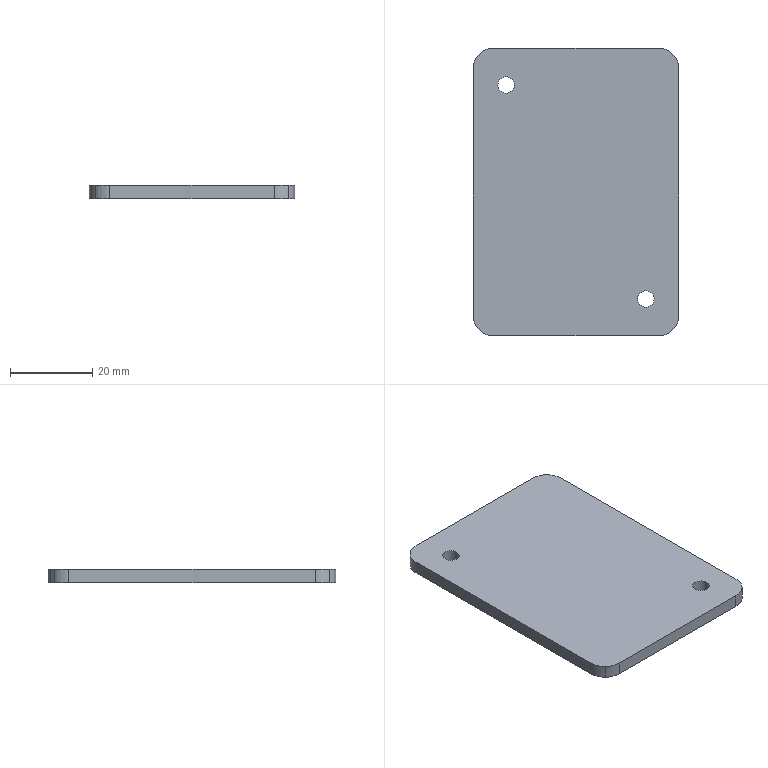Part | STEP file | DCV-000-017 | 1 solid | 18 faces | box 50 x 70 x 3.2 mm | volume 11051 mm3 | cylinder 12 | plane 6 | commonest cylinder face diameters 10 x8 4 x4
STEP:
#1=CARTESIAN_POINT('',(0.,0.,0.));
#2=DIRECTION('',(0.,0.,1.));
#3=DIRECTION('',(1.,0.,0.));
#4=AXIS2_PLACEMENT_3D('',#1,#2,#3);
#5=CARTESIAN_POINT('',(20.,0.,0.));
#6=VERTEX_POINT('',#5);
#7=CARTESIAN_POINT('',(23.536,1.464,0.));
#8=VERTEX_POINT('',#7);
#9=CARTESIAN_POINT('',(20.,5.,0.));
#10=DIRECTION('',(0.,0.,1.));
#11=DIRECTION('',(0.7071,-0.7071,0.));
#12=AXIS2_PLACEMENT_3D('',#9,#10,#11);
#13=CIRCLE('',#12,5.);
#14=CARTESIAN_POINT('',(20.,5.,0.));
#15=DIRECTION('',(0.,0.,1.));
#16=DIRECTION('',(0.7071,-0.7071,0.));
#17=AXIS2_PLACEMENT_3D('',#14,#15,#16);
#18=CYLINDRICAL_SURFACE('',#17,5.);
#19=CARTESIAN_POINT('',(0.,0.));
#20=DIRECTION('',(1.,0.));
#21=VECTOR('',#20,1.);
#22=LINE('',#19,#21);
#23=(GEOMETRIC_REPRESENTATION_CONTEXT(2)PARAMETRIC_REPRESENTATION_CONTEXT()REPRESENTATION_CONTEXT('',''));
#24=DEFINITIONAL_REPRESENTATION('',(#22),#23);
#25=PCURVE('',#18,#24);
#26=CARTESIAN_POINT('',(0.,35.,0.));
#27=DIRECTION('',(0.,0.,1.));
#28=DIRECTION('',(1.,0.,0.));
#29=AXIS2_PLACEMENT_3D('',#26,#27,#28);
#30=PLANE('',#29);
#31=CARTESIAN_POINT('',(20.,-30.));
#32=DIRECTION('',(0.7071,-0.7071));
#33=AXIS2_PLACEMENT_2D('',#31,#32);
#34=CIRCLE('',#33,5.);
#35=(GEOMETRIC_REPRESENTATION_CONTEXT(2)PARAMETRIC_REPRESENTATION_CONTEXT()REPRESENTATION_CONTEXT('',''));
#36=DEFINITIONAL_REPRESENTATION('',(#34),#35);
#37=PCURVE('',#30,#36);
#38=SURFACE_CURVE('',#13,(#25,#37),.PCURVE_S1.);
#39=EDGE_CURVE('',#6,#8,#38,.T.);
#40=ORIENTED_EDGE('',*,*,#39,.T.);
#41=CARTESIAN_POINT('',(23.536,1.464,3.2));
#42=VERTEX_POINT('',#41);
#43=CARTESIAN_POINT('',(23.536,1.464,0.));
#44=DIRECTION('',(0.,0.,1.));
#45=VECTOR('',#44,1.);
#46=LINE('',#43,#45);
#47=CARTESIAN_POINT('',(6.283,0.));
#48=DIRECTION('',(0.,1.));
#49=VECTOR('',#48,1.);
#50=LINE('',#47,#49);
#51=(GEOMETRIC_REPRESENTATION_CONTEXT(2)PARAMETRIC_REPRESENTATION_CONTEXT()REPRESENTATION_CONTEXT('',''));
#52=DEFINITIONAL_REPRESENTATION('',(#50),#51);
#53=PCURVE('',#18,#52);
#54=CARTESIAN_POINT('',(20.,5.,0.));
#55=DIRECTION('',(0.,0.,1.));
#56=DIRECTION('',(0.7071,-0.7071,0.));
#57=AXIS2_PLACEMENT_3D('',#54,#55,#56);
#58=CYLINDRICAL_SURFACE('',#57,5.);
#59=CARTESIAN_POINT('',(0.,0.));
#60=DIRECTION('',(0.,1.));
#61=VECTOR('',#60,1.);
#62=LINE('',#59,#61);
#63=(GEOMETRIC_REPRESENTATION_CONTEXT(2)PARAMETRIC_REPRESENTATION_CONTEXT()REPRESENTATION_CONTEXT('',''));
#64=DEFINITIONAL_REPRESENTATION('',(#62),#63);
#65=PCURVE('',#58,#64);
#66=SURFACE_CURVE('',#46,(#53,#65),.PCURVE_S1.);
#67=EDGE_CURVE('',#8,#42,#66,.T.);
#68=ORIENTED_EDGE('',*,*,#67,.T.);
#69=CARTESIAN_POINT('',(20.,0.,3.2));
#70=VERTEX_POINT('',#69);
#71=CARTESIAN_POINT('',(20.,5.,3.2));
#72=DIRECTION('',(0.,0.,-1.));
#73=DIRECTION('',(0.7071,-0.7071,0.));
#74=AXIS2_PLACEMENT_3D('',#71,#72,#73);
#75=CIRCLE('',#74,5.);
#76=CARTESIAN_POINT('',(6.283,3.2));
#77=DIRECTION('',(-1.,0.));
#78=VECTOR('',#77,1.);
#79=LINE('',#76,#78);
#80=(GEOMETRIC_REPRESENTATION_CONTEXT(2)PARAMETRIC_REPRESENTATION_CONTEXT()REPRESENTATION_CONTEXT('',''));
#81=DEFINITIONAL_REPRESENTATION('',(#79),#80);
#82=PCURVE('',#18,#81);
#83=CARTESIAN_POINT('',(0.,35.,3.2));
#84=DIRECTION('',(0.,0.,1.));
#85=DIRECTION('',(1.,0.,0.));
#86=AXIS2_PLACEMENT_3D('',#83,#84,#85);
#87=PLANE('',#86);
#88=CARTESIAN_POINT('',(23.536,-33.536));
#89=CARTESIAN_POINT('',(17.412,-39.659));
#90=CARTESIAN_POINT('',(15.17,-31.294));
#91=CARTESIAN_POINT('',(12.929,-22.929));
#92=CARTESIAN_POINT('',(21.294,-25.17));
#93=CARTESIAN_POINT('',(29.659,-27.412));
#94=CARTESIAN_POINT('',(23.536,-33.536));
#95=(BOUNDED_CURVE()B_SPLINE_CURVE(2,(#88,#89,#90,#91,#92,#93,#94),.UNSPECIFIED.,.T.,.F.)B_SPLINE_CURVE_WITH_KNOTS((1,2,2,2,2,1),(-2.094,0.,2.094,4.189,6.283,8.378),.UNSPECIFIED.)CURVE()GEOMETRIC_REPRESENTATION_ITEM()RATIONAL_B_SPLINE_CURVE((1.,0.5,1.,0.5,1.,0.5,1.))REPRESENTATION_ITEM(''));
#96=(GEOMETRIC_REPRESENTATION_CONTEXT(2)PARAMETRIC_REPRESENTATION_CONTEXT()REPRESENTATION_CONTEXT('',''));
#97=DEFINITIONAL_REPRESENTATION('',(#95),#96);
#98=PCURVE('',#87,#97);
#99=SURFACE_CURVE('',#75,(#82,#98),.PCURVE_S1.);
#100=EDGE_CURVE('',#42,#70,#99,.T.);
#101=ORIENTED_EDGE('',*,*,#100,.T.);
#102=CARTESIAN_POINT('',(20.,0.,0.));
#103=DIRECTION('',(0.,0.,-1.));
#104=VECTOR('',#103,1.);
#105=LINE('',#102,#104);
#106=CARTESIAN_POINT('',(5.498,0.));
#107=DIRECTION('',(0.,-1.));
#108=VECTOR('',#107,1.);
#109=LINE('',#106,#108);
#110=(GEOMETRIC_REPRESENTATION_CONTEXT(2)PARAMETRIC_REPRESENTATION_CONTEXT()REPRESENTATION_CONTEXT('',''));
#111=DEFINITIONAL_REPRESENTATION('',(#109),#110);
#112=PCURVE('',#18,#111);
#113=CARTESIAN_POINT('',(-25.,0.,0.));
#114=DIRECTION('',(0.,-1.,0.));
#115=DIRECTION('',(0.,0.,-1.));
#116=AXIS2_PLACEMENT_3D('',#113,#114,#115);
#117=PLANE('',#116);
#118=CARTESIAN_POINT('',(0.,45.));
#119=DIRECTION('',(1.,0.));
#120=VECTOR('',#119,1.);
#121=LINE('',#118,#120);
#122=(GEOMETRIC_REPRESENTATION_CONTEXT(2)PARAMETRIC_REPRESENTATION_CONTEXT()REPRESENTATION_CONTEXT('',''));
#123=DEFINITIONAL_REPRESENTATION('',(#121),#122);
#124=PCURVE('',#117,#123);
#125=SURFACE_CURVE('',#105,(#112,#124),.PCURVE_S1.);
#126=EDGE_CURVE('',#70,#6,#125,.T.);
#127=ORIENTED_EDGE('',*,*,#126,.T.);
#128=EDGE_LOOP('',(#40,#68,#101,#127));
#129=FACE_BOUND('',#128,.T.);
#130=ADVANCED_FACE('',(#129),#18,.T.);
#131=CARTESIAN_POINT('',(-25.,5.,0.));
#132=VERTEX_POINT('',#131);
#133=CARTESIAN_POINT('',(-23.536,1.464,0.));
#134=VERTEX_POINT('',#133);
#135=CARTESIAN_POINT('',(-20.,5.,0.));
#136=DIRECTION('',(0.,0.,1.));
#137=DIRECTION('',(-0.7071,-0.7071,0.));
#138=AXIS2_PLACEMENT_3D('',#135,#136,#137);
#139=CIRCLE('',#138,5.);
#140=CARTESIAN_POINT('',(-20.,5.,0.));
#141=DIRECTION('',(0.,0.,1.));
#142=DIRECTION('',(-0.7071,-0.7071,0.));
#143=AXIS2_PLACEMENT_3D('',#140,#141,#142);
#144=CYLINDRICAL_SURFACE('',#143,5.);
#145=CARTESIAN_POINT('',(0.,0.));
#146=DIRECTION('',(1.,0.));
#147=VECTOR('',#146,1.);
#148=LINE('',#145,#147);
#149=(GEOMETRIC_REPRESENTATION_CONTEXT(2)PARAMETRIC_REPRESENTATION_CONTEXT()REPRESENTATION_CONTEXT('',''));
#150=DEFINITIONAL_REPRESENTATION('',(#148),#149);
#151=PCURVE('',#144,#150);
#152=CARTESIAN_POINT('',(-20.,-30.));
#153=DIRECTION('',(-0.7071,-0.7071));
#154=AXIS2_PLACEMENT_2D('',#152,#153);
#155=CIRCLE('',#154,5.);
#156=(GEOMETRIC_REPRESENTATION_CONTEXT(2)PARAMETRIC_REPRESENTATION_CONTEXT()REPRESENTATION_CONTEXT('',''));
#157=DEFINITIONAL_REPRESENTATION('',(#155),#156);
#158=PCURVE('',#30,#157);
#159=SURFACE_CURVE('',#139,(#151,#158),.PCURVE_S1.);
#160=EDGE_CURVE('',#132,#134,#159,.T.);
#161=ORIENTED_EDGE('',*,*,#160,.T.);
#162=CARTESIAN_POINT('',(-23.536,1.464,3.2));
#163=VERTEX_POINT('',#162);
#164=CARTESIAN_POINT('',(-23.536,1.464,0.));
#165=DIRECTION('',(0.,0.,1.));
#166=VECTOR('',#165,1.);
#167=LINE('',#164,#166);
#168=CARTESIAN_POINT('',(6.283,0.));
#169=DIRECTION('',(0.,1.));
#170=VECTOR('',#169,1.);
#171=LINE('',#168,#170);
#172=(GEOMETRIC_REPRESENTATION_CONTEXT(2)PARAMETRIC_REPRESENTATION_CONTEXT()REPRESENTATION_CONTEXT('',''));
#173=DEFINITIONAL_REPRESENTATION('',(#171),#172);
#174=PCURVE('',#144,#173);
#175=CARTESIAN_POINT('',(-20.,5.,0.));
#176=DIRECTION('',(0.,0.,1.));
#177=DIRECTION('',(-0.7071,-0.7071,0.));
#178=AXIS2_PLACEMENT_3D('',#175,#176,#177);
#179=CYLINDRICAL_SURFACE('',#178,5.);
#180=CARTESIAN_POINT('',(0.,0.));
#181=DIRECTION('',(0.,1.));
#182=VECTOR('',#181,1.);
#183=LINE('',#180,#182);
#184=(GEOMETRIC_REPRESENTATION_CONTEXT(2)PARAMETRIC_REPRESENTATION_CONTEXT()REPRESENTATION_CONTEXT('',''));
#185=DEFINITIONAL_REPRESENTATION('',(#183),#184);
#186=PCURVE('',#179,#185);
#187=SURFACE_CURVE('',#167,(#174,#186),.PCURVE_S1.);
#188=EDGE_CURVE('',#134,#163,#187,.T.);
#189=ORIENTED_EDGE('',*,*,#188,.T.);
#190=CARTESIAN_POINT('',(-25.,5.,3.2));
#191=VERTEX_POINT('',#190);
#192=CARTESIAN_POINT('',(-20.,5.,3.2));
#193=DIRECTION('',(0.,0.,-1.));
#194=DIRECTION('',(-0.7071,-0.7071,0.));
#195=AXIS2_PLACEMENT_3D('',#192,#193,#194);
#196=CIRCLE('',#195,5.);
#197=CARTESIAN_POINT('',(6.283,3.2));
#198=DIRECTION('',(-1.,0.));
#199=VECTOR('',#198,1.);
#200=LINE('',#197,#199);
#201=(GEOMETRIC_REPRESENTATION_CONTEXT(2)PARAMETRIC_REPRESENTATION_CONTEXT()REPRESENTATION_CONTEXT('',''));
#202=DEFINITIONAL_REPRESENTATION('',(#200),#201);
#203=PCURVE('',#144,#202);
#204=CARTESIAN_POINT('',(-23.536,-33.536));
#205=CARTESIAN_POINT('',(-29.659,-27.412));
#206=CARTESIAN_POINT('',(-21.294,-25.17));
#207=CARTESIAN_POINT('',(-12.929,-22.929));
#208=CARTESIAN_POINT('',(-15.17,-31.294));
#209=CARTESIAN_POINT('',(-17.412,-39.659));
#210=CARTESIAN_POINT('',(-23.536,-33.536));
#211=(BOUNDED_CURVE()B_SPLINE_CURVE(2,(#204,#205,#206,#207,#208,#209,#210),.UNSPECIFIED.,.T.,.F.)B_SPLINE_CURVE_WITH_KNOTS((1,2,2,2,2,1),(-2.094,0.,2.094,4.189,6.283,8.378),.UNSPECIFIED.)CURVE()GEOMETRIC_REPRESENTATION_ITEM()RATIONAL_B_SPLINE_CURVE((1.,0.5,1.,0.5,1.,0.5,1.))REPRESENTATION_ITEM(''));
#212=(GEOMETRIC_REPRESENTATION_CONTEXT(2)PARAMETRIC_REPRESENTATION_CONTEXT()REPRESENTATION_CONTEXT('',''));
#213=DEFINITIONAL_REPRESENTATION('',(#211),#212);
#214=PCURVE('',#87,#213);
#215=SURFACE_CURVE('',#196,(#203,#214),.PCURVE_S1.);
#216=EDGE_CURVE('',#163,#191,#215,.T.);
#217=ORIENTED_EDGE('',*,*,#216,.T.);
#218=CARTESIAN_POINT('',(-25.,5.,0.));
#219=DIRECTION('',(0.,0.,-1.));
#220=VECTOR('',#219,1.);
#221=LINE('',#218,#220);
#222=CARTESIAN_POINT('',(5.498,0.));
#223=DIRECTION('',(0.,-1.));
#224=VECTOR('',#223,1.);
#225=LINE('',#222,#224);
#226=(GEOMETRIC_REPRESENTATION_CONTEXT(2)PARAMETRIC_REPRESENTATION_CONTEXT()REPRESENTATION_CONTEXT('',''));
#227=DEFINITIONAL_REPRESENTATION('',(#225),#226);
#228=PCURVE('',#144,#227);
#229=CARTESIAN_POINT('',(-25.,70.,0.));
#230=DIRECTION('',(-1.,0.,0.));
#231=DIRECTION('',(0.,0.,1.));
#232=AXIS2_PLACEMENT_3D('',#229,#230,#231);
#233=PLANE('',#232);
#234=CARTESIAN_POINT('',(0.,-65.));
#235=DIRECTION('',(-1.,0.));
#236=VECTOR('',#235,1.);
#237=LINE('',#234,#236);
#238=(GEOMETRIC_REPRESENTATION_CONTEXT(2)PARAMETRIC_REPRESENTATION_CONTEXT()REPRESENTATION_CONTEXT('',''));
#239=DEFINITIONAL_REPRESENTATION('',(#237),#238);
#240=PCURVE('',#233,#239);
#241=SURFACE_CURVE('',#221,(#228,#240),.PCURVE_S1.);
#242=EDGE_CURVE('',#191,#132,#241,.T.);
#243=ORIENTED_EDGE('',*,*,#242,.T.);
#244=EDGE_LOOP('',(#161,#189,#217,#243));
#245=FACE_BOUND('',#244,.T.);
#246=ADVANCED_FACE('',(#245),#144,.T.);
#247=CARTESIAN_POINT('',(-20.,70.,0.));
#248=VERTEX_POINT('',#247);
#249=CARTESIAN_POINT('',(-23.536,68.536,0.));
#250=VERTEX_POINT('',#249);
#251=CARTESIAN_POINT('',(-20.,65.,0.));
#252=DIRECTION('',(0.,0.,1.));
#253=DIRECTION('',(-0.7071,0.7071,0.));
#254=AXIS2_PLACEMENT_3D('',#251,#252,#253);
#255=CIRCLE('',#254,5.);
#256=CARTESIAN_POINT('',(-20.,65.,0.));
#257=DIRECTION('',(0.,0.,1.));
#258=DIRECTION('',(-0.7071,0.7071,0.));
#259=AXIS2_PLACEMENT_3D('',#256,#257,#258);
#260=CYLINDRICAL_SURFACE('',#259,5.);
#261=CARTESIAN_POINT('',(0.,0.));
#262=DIRECTION('',(1.,0.));
#263=VECTOR('',#262,1.);
#264=LINE('',#261,#263);
#265=(GEOMETRIC_REPRESENTATION_CONTEXT(2)PARAMETRIC_REPRESENTATION_CONTEXT()REPRESENTATION_CONTEXT('',''));
#266=DEFINITIONAL_REPRESENTATION('',(#264),#265);
#267=PCURVE('',#260,#266);
#268=CARTESIAN_POINT('',(-20.,30.));
#269=DIRECTION('',(-0.7071,0.7071));
#270=AXIS2_PLACEMENT_2D('',#268,#269);
#271=CIRCLE('',#270,5.);
#272=(GEOMETRIC_REPRESENTATION_CONTEXT(2)PARAMETRIC_REPRESENTATION_CONTEXT()REPRESENTATION_CONTEXT('',''));
#273=DEFINITIONAL_REPRESENTATION('',(#271),#272);
#274=PCURVE('',#30,#273);
#275=SURFACE_CURVE('',#255,(#267,#274),.PCURVE_S1.);
#276=EDGE_CURVE('',#248,#250,#275,.T.);
#277=ORIENTED_EDGE('',*,*,#276,.T.);
#278=CARTESIAN_POINT('',(-23.536,68.536,3.2));
#279=VERTEX_POINT('',#278);
#280=CARTESIAN_POINT('',(-23.536,68.536,0.));
#281=DIRECTION('',(0.,0.,1.));
#282=VECTOR('',#281,1.);
#283=LINE('',#280,#282);
#284=CARTESIAN_POINT('',(6.283,0.));
#285=DIRECTION('',(0.,1.));
#286=VECTOR('',#285,1.);
#287=LINE('',#284,#286);
#288=(GEOMETRIC_REPRESENTATION_CONTEXT(2)PARAMETRIC_REPRESENTATION_CONTEXT()REPRESENTATION_CONTEXT('',''));
#289=DEFINITIONAL_REPRESENTATION('',(#287),#288);
#290=PCURVE('',#260,#289);
#291=CARTESIAN_POINT('',(-20.,65.,0.));
#292=DIRECTION('',(0.,0.,1.));
#293=DIRECTION('',(-0.7071,0.7071,0.));
#294=AXIS2_PLACEMENT_3D('',#291,#292,#293);
#295=CYLINDRICAL_SURFACE('',#294,5.);
#296=CARTESIAN_POINT('',(0.,0.));
#297=DIRECTION('',(0.,1.));
#298=VECTOR('',#297,1.);
#299=LINE('',#296,#298);
#300=(GEOMETRIC_REPRESENTATION_CONTEXT(2)PARAMETRIC_REPRESENTATION_CONTEXT()REPRESENTATION_CONTEXT('',''));
#301=DEFINITIONAL_REPRESENTATION('',(#299),#300);
#302=PCURVE('',#295,#301);
#303=SURFACE_CURVE('',#283,(#290,#302),.PCURVE_S1.);
#304=EDGE_CURVE('',#250,#279,#303,.T.);
#305=ORIENTED_EDGE('',*,*,#304,.T.);
#306=CARTESIAN_POINT('',(-20.,70.,3.2));
#307=VERTEX_POINT('',#306);
#308=CARTESIAN_POINT('',(-20.,65.,3.2));
#309=DIRECTION('',(0.,0.,-1.));
#310=DIRECTION('',(-0.7071,0.7071,0.));
#311=AXIS2_PLACEMENT_3D('',#308,#309,#310);
#312=CIRCLE('',#311,5.);
#313=CARTESIAN_POINT('',(6.283,3.2));
#314=DIRECTION('',(-1.,0.));
#315=VECTOR('',#314,1.);
#316=LINE('',#313,#315);
#317=(GEOMETRIC_REPRESENTATION_CONTEXT(2)PARAMETRIC_REPRESENTATION_CONTEXT()REPRESENTATION_CONTEXT('',''));
#318=DEFINITIONAL_REPRESENTATION('',(#316),#317);
#319=PCURVE('',#260,#318);
#320=CARTESIAN_POINT('',(-23.536,33.536));
#321=CARTESIAN_POINT('',(-17.412,39.659));
#322=CARTESIAN_POINT('',(-15.17,31.294));
#323=CARTESIAN_POINT('',(-12.929,22.929));
#324=CARTESIAN_POINT('',(-21.294,25.17));
#325=CARTESIAN_POINT('',(-29.659,27.412));
#326=CARTESIAN_POINT('',(-23.536,33.536));
#327=(BOUNDED_CURVE()B_SPLINE_CURVE(2,(#320,#321,#322,#323,#324,#325,#326),.UNSPECIFIED.,.T.,.F.)B_SPLINE_CURVE_WITH_KNOTS((1,2,2,2,2,1),(-2.094,0.,2.094,4.189,6.283,8.378),.UNSPECIFIED.)CURVE()GEOMETRIC_REPRESENTATION_ITEM()RATIONAL_B_SPLINE_CURVE((1.,0.5,1.,0.5,1.,0.5,1.))REPRESENTATION_ITEM(''));
#328=(GEOMETRIC_REPRESENTATION_CONTEXT(2)PARAMETRIC_REPRESENTATION_CONTEXT()REPRESENTATION_CONTEXT('',''));
#329=DEFINITIONAL_REPRESENTATION('',(#327),#328);
#330=PCURVE('',#87,#329);
#331=SURFACE_CURVE('',#312,(#319,#330),.PCURVE_S1.);
#332=EDGE_CURVE('',#279,#307,#331,.T.);
#333=ORIENTED_EDGE('',*,*,#332,.T.);
#334=CARTESIAN_POINT('',(-20.,70.,0.));
#335=DIRECTION('',(0.,0.,-1.));
#336=VECTOR('',#335,1.);
#337=LINE('',#334,#336);
#338=CARTESIAN_POINT('',(5.498,0.));
#339=DIRECTION('',(0.,-1.));
#340=VECTOR('',#339,1.);
#341=LINE('',#338,#340);
#342=(GEOMETRIC_REPRESENTATION_CONTEXT(2)PARAMETRIC_REPRESENTATION_CONTEXT()REPRESENTATION_CONTEXT('',''));
#343=DEFINITIONAL_REPRESENTATION('',(#341),#342);
#344=PCURVE('',#260,#343);
#345=CARTESIAN_POINT('',(25.,70.,0.));
#346=DIRECTION('',(0.,1.,0.));
#347=DIRECTION('',(1.,0.,0.));
#348=AXIS2_PLACEMENT_3D('',#345,#346,#347);
#349=PLANE('',#348);
#350=CARTESIAN_POINT('',(-45.,0.));
#351=DIRECTION('',(0.,1.));
#352=VECTOR('',#351,1.);
#353=LINE('',#350,#352);
#354=(GEOMETRIC_REPRESENTATION_CONTEXT(2)PARAMETRIC_REPRESENTATION_CONTEXT()REPRESENTATION_CONTEXT('',''));
#355=DEFINITIONAL_REPRESENTATION('',(#353),#354);
#356=PCURVE('',#349,#355);
#357=SURFACE_CURVE('',#337,(#344,#356),.PCURVE_S1.);
#358=EDGE_CURVE('',#307,#248,#357,.T.);
#359=ORIENTED_EDGE('',*,*,#358,.T.);
#360=EDGE_LOOP('',(#277,#305,#333,#359));
#361=FACE_BOUND('',#360,.T.);
#362=ADVANCED_FACE('',(#361),#260,.T.);
#363=CARTESIAN_POINT('',(25.,65.,0.));
#364=VERTEX_POINT('',#363);
#365=CARTESIAN_POINT('',(23.536,68.536,0.));
#366=VERTEX_POINT('',#365);
#367=CARTESIAN_POINT('',(20.,65.,0.));
#368=DIRECTION('',(0.,0.,1.));
#369=DIRECTION('',(0.7071,0.7071,0.));
#370=AXIS2_PLACEMENT_3D('',#367,#368,#369);
#371=CIRCLE('',#370,5.);
#372=CARTESIAN_POINT('',(20.,65.,0.));
#373=DIRECTION('',(0.,0.,1.));
#374=DIRECTION('',(0.7071,0.7071,0.));
#375=AXIS2_PLACEMENT_3D('',#372,#373,#374);
#376=CYLINDRICAL_SURFACE('',#375,5.);
#377=CARTESIAN_POINT('',(0.,0.));
#378=DIRECTION('',(1.,0.));
#379=VECTOR('',#378,1.);
#380=LINE('',#377,#379);
#381=(GEOMETRIC_REPRESENTATION_CONTEXT(2)PARAMETRIC_REPRESENTATION_CONTEXT()REPRESENTATION_CONTEXT('',''));
#382=DEFINITIONAL_REPRESENTATION('',(#380),#381);
#383=PCURVE('',#376,#382);
#384=CARTESIAN_POINT('',(20.,30.));
#385=DIRECTION('',(0.7071,0.7071));
#386=AXIS2_PLACEMENT_2D('',#384,#385);
#387=CIRCLE('',#386,5.);
#388=(GEOMETRIC_REPRESENTATION_CONTEXT(2)PARAMETRIC_REPRESENTATION_CONTEXT()REPRESENTATION_CONTEXT('',''));
#389=DEFINITIONAL_REPRESENTATION('',(#387),#388);
#390=PCURVE('',#30,#389);
#391=SURFACE_CURVE('',#371,(#383,#390),.PCURVE_S1.);
#392=EDGE_CURVE('',#364,#366,#391,.T.);
#393=ORIENTED_EDGE('',*,*,#392,.T.);
#394=CARTESIAN_POINT('',(23.536,68.536,3.2));
#395=VERTEX_POINT('',#394);
#396=CARTESIAN_POINT('',(23.536,68.536,0.));
#397=DIRECTION('',(0.,0.,1.));
#398=VECTOR('',#397,1.);
#399=LINE('',#396,#398);
#400=CARTESIAN_POINT('',(6.283,0.));
#401=DIRECTION('',(0.,1.));
#402=VECTOR('',#401,1.);
#403=LINE('',#400,#402);
#404=(GEOMETRIC_REPRESENTATION_CONTEXT(2)PARAMETRIC_REPRESENTATION_CONTEXT()REPRESENTATION_CONTEXT('',''));
#405=DEFINITIONAL_REPRESENTATION('',(#403),#404);
#406=PCURVE('',#376,#405);
#407=CARTESIAN_POINT('',(20.,65.,0.));
#408=DIRECTION('',(0.,0.,1.));
#409=DIRECTION('',(0.7071,0.7071,0.));
#410=AXIS2_PLACEMENT_3D('',#407,#408,#409);
#411=CYLINDRICAL_SURFACE('',#410,5.);
#412=CARTESIAN_POINT('',(0.,0.));
#413=DIRECTION('',(0.,1.));
#414=VECTOR('',#413,1.);
#415=LINE('',#412,#414);
#416=(GEOMETRIC_REPRESENTATION_CONTEXT(2)PARAMETRIC_REPRESENTATION_CONTEXT()REPRESENTATION_CONTEXT('',''));
#417=DEFINITIONAL_REPRESENTATION('',(#415),#416);
#418=PCURVE('',#411,#417);
#419=SURFACE_CURVE('',#399,(#406,#418),.PCURVE_S1.);
#420=EDGE_CURVE('',#366,#395,#419,.T.);
#421=ORIENTED_EDGE('',*,*,#420,.T.);
#422=CARTESIAN_POINT('',(25.,65.,3.2));
#423=VERTEX_POINT('',#422);
#424=CARTESIAN_POINT('',(20.,65.,3.2));
#425=DIRECTION('',(0.,0.,-1.));
#426=DIRECTION('',(0.7071,0.7071,0.));
#427=AXIS2_PLACEMENT_3D('',#424,#425,#426);
#428=CIRCLE('',#427,5.);
#429=CARTESIAN_POINT('',(6.283,3.2));
#430=DIRECTION('',(-1.,0.));
#431=VECTOR('',#430,1.);
#432=LINE('',#429,#431);
#433=(GEOMETRIC_REPRESENTATION_CONTEXT(2)PARAMETRIC_REPRESENTATION_CONTEXT()REPRESENTATION_CONTEXT('',''));
#434=DEFINITIONAL_REPRESENTATION('',(#432),#433);
#435=PCURVE('',#376,#434);
#436=CARTESIAN_POINT('',(23.536,33.536));
#437=CARTESIAN_POINT('',(29.659,27.412));
#438=CARTESIAN_POINT('',(21.294,25.17));
#439=CARTESIAN_POINT('',(12.929,22.929));
#440=CARTESIAN_POINT('',(15.17,31.294));
#441=CARTESIAN_POINT('',(17.412,39.659));
#442=CARTESIAN_POINT('',(23.536,33.536));
#443=(BOUNDED_CURVE()B_SPLINE_CURVE(2,(#436,#437,#438,#439,#440,#441,#442),.UNSPECIFIED.,.T.,.F.)B_SPLINE_CURVE_WITH_KNOTS((1,2,2,2,2,1),(-2.094,0.,2.094,4.189,6.283,8.378),.UNSPECIFIED.)CURVE()GEOMETRIC_REPRESENTATION_ITEM()RATIONAL_B_SPLINE_CURVE((1.,0.5,1.,0.5,1.,0.5,1.))REPRESENTATION_ITEM(''));
#444=(GEOMETRIC_REPRESENTATION_CONTEXT(2)PARAMETRIC_REPRESENTATION_CONTEXT()REPRESENTATION_CONTEXT('',''));
#445=DEFINITIONAL_REPRESENTATION('',(#443),#444);
#446=PCURVE('',#87,#445);
#447=SURFACE_CURVE('',#428,(#435,#446),.PCURVE_S1.);
#448=EDGE_CURVE('',#395,#423,#447,.T.);
#449=ORIENTED_EDGE('',*,*,#448,.T.);
#450=CARTESIAN_POINT('',(25.,65.,0.));
#451=DIRECTION('',(0.,0.,-1.));
#452=VECTOR('',#451,1.);
#453=LINE('',#450,#452);
#454=CARTESIAN_POINT('',(5.498,0.));
#455=DIRECTION('',(0.,-1.));
#456=VECTOR('',#455,1.);
#457=LINE('',#454,#456);
#458=(GEOMETRIC_REPRESENTATION_CONTEXT(2)PARAMETRIC_REPRESENTATION_CONTEXT()REPRESENTATION_CONTEXT('',''));
#459=DEFINITIONAL_REPRESENTATION('',(#457),#458);
#460=PCURVE('',#376,#459);
#461=CARTESIAN_POINT('',(25.,0.,0.));
#462=DIRECTION('',(1.,0.,0.));
#463=DIRECTION('',(0.,-1.,0.));
#464=AXIS2_PLACEMENT_3D('',#461,#462,#463);
#465=PLANE('',#464);
#466=CARTESIAN_POINT('',(-65.,0.));
#467=DIRECTION('',(0.,1.));
#468=VECTOR('',#467,1.);
#469=LINE('',#466,#468);
#470=(GEOMETRIC_REPRESENTATION_CONTEXT(2)PARAMETRIC_REPRESENTATION_CONTEXT()REPRESENTATION_CONTEXT('',''));
#471=DEFINITIONAL_REPRESENTATION('',(#469),#470);
#472=PCURVE('',#465,#471);
#473=SURFACE_CURVE('',#453,(#460,#472),.PCURVE_S1.);
#474=EDGE_CURVE('',#423,#364,#473,.T.);
#475=ORIENTED_EDGE('',*,*,#474,.T.);
#476=EDGE_LOOP('',(#393,#421,#449,#475));
#477=FACE_BOUND('',#476,.T.);
#478=ADVANCED_FACE('',(#477),#376,.T.);
#479=CARTESIAN_POINT('',(19.,9.,0.));
#480=VERTEX_POINT('',#479);
#481=CARTESIAN_POINT('',(19.,9.,3.2));
#482=VERTEX_POINT('',#481);
#483=CARTESIAN_POINT('',(19.,9.,86.083));
#484=DIRECTION('',(0.,0.,1.));
#485=VECTOR('',#484,1.);
#486=LINE('',#483,#485);
#487=CARTESIAN_POINT('',(17.,9.,86.083));
#488=DIRECTION('',(0.,0.,1.));
#489=DIRECTION('',(1.,0.,0.));
#490=AXIS2_PLACEMENT_3D('',#487,#488,#489);
#491=CYLINDRICAL_SURFACE('',#490,2.);
#492=CARTESIAN_POINT('',(6.283,0.));
#493=DIRECTION('',(0.,1.));
#494=VECTOR('',#493,1.);
#495=LINE('',#492,#494);
#496=(GEOMETRIC_REPRESENTATION_CONTEXT(2)PARAMETRIC_REPRESENTATION_CONTEXT()REPRESENTATION_CONTEXT('',''));
#497=DEFINITIONAL_REPRESENTATION('',(#495),#496);
#498=PCURVE('',#491,#497);
#499=CARTESIAN_POINT('',(17.,9.,86.083));
#500=DIRECTION('',(0.,0.,1.));
#501=DIRECTION('',(1.,0.,0.));
#502=AXIS2_PLACEMENT_3D('',#499,#500,#501);
#503=CYLINDRICAL_SURFACE('',#502,2.);
#504=CARTESIAN_POINT('',(0.,0.));
#505=DIRECTION('',(0.,1.));
#506=VECTOR('',#505,1.);
#507=LINE('',#504,#506);
#508=(GEOMETRIC_REPRESENTATION_CONTEXT(2)PARAMETRIC_REPRESENTATION_CONTEXT()REPRESENTATION_CONTEXT('',''));
#509=DEFINITIONAL_REPRESENTATION('',(#507),#508);
#510=PCURVE('',#503,#509);
#511=SURFACE_CURVE('',#486,(#498,#510),.PCURVE_S1.);
#512=EDGE_CURVE('',#480,#482,#511,.T.);
#513=ORIENTED_EDGE('',*,*,#512,.T.);
#514=CARTESIAN_POINT('',(15.,9.,3.2));
#515=VERTEX_POINT('',#514);
#516=CARTESIAN_POINT('',(17.,9.,3.2));
#517=DIRECTION('',(0.,0.,-1.));
#518=DIRECTION('',(1.,0.,0.));
#519=AXIS2_PLACEMENT_3D('',#516,#517,#518);
#520=CIRCLE('',#519,2.);
#521=CARTESIAN_POINT('',(6.283,-82.883));
#522=DIRECTION('',(-1.,0.));
#523=VECTOR('',#522,1.);
#524=LINE('',#521,#523);
#525=(GEOMETRIC_REPRESENTATION_CONTEXT(2)PARAMETRIC_REPRESENTATION_CONTEXT()REPRESENTATION_CONTEXT('',''));
#526=DEFINITIONAL_REPRESENTATION('',(#524),#525);
#527=PCURVE('',#491,#526);
#528=CARTESIAN_POINT('',(19.,-26.));
#529=CARTESIAN_POINT('',(19.,-29.464));
#530=CARTESIAN_POINT('',(16.,-27.732));
#531=CARTESIAN_POINT('',(13.,-26.));
#532=CARTESIAN_POINT('',(16.,-24.268));
#533=CARTESIAN_POINT('',(19.,-22.536));
#534=CARTESIAN_POINT('',(19.,-26.));
#535=(BOUNDED_CURVE()B_SPLINE_CURVE(2,(#528,#529,#530,#531,#532,#533,#534),.UNSPECIFIED.,.T.,.F.)B_SPLINE_CURVE_WITH_KNOTS((1,2,2,2,2,1),(-2.094,0.,2.094,4.189,6.283,8.378),.UNSPECIFIED.)CURVE()GEOMETRIC_REPRESENTATION_ITEM()RATIONAL_B_SPLINE_CURVE((1.,0.5,1.,0.5,1.,0.5,1.))REPRESENTATION_ITEM(''));
#536=(GEOMETRIC_REPRESENTATION_CONTEXT(2)PARAMETRIC_REPRESENTATION_CONTEXT()REPRESENTATION_CONTEXT('',''));
#537=DEFINITIONAL_REPRESENTATION('',(#535),#536);
#538=PCURVE('',#87,#537);
#539=SURFACE_CURVE('',#520,(#527,#538),.PCURVE_S1.);
#540=EDGE_CURVE('',#482,#515,#539,.T.);
#541=ORIENTED_EDGE('',*,*,#540,.T.);
#542=CARTESIAN_POINT('',(15.,9.,0.));
#543=VERTEX_POINT('',#542);
#544=CARTESIAN_POINT('',(15.,9.,86.083));
#545=DIRECTION('',(0.,0.,1.));
#546=VECTOR('',#545,1.);
#547=LINE('',#544,#546);
#548=CARTESIAN_POINT('',(3.142,0.));
#549=DIRECTION('',(0.,1.));
#550=VECTOR('',#549,1.);
#551=LINE('',#548,#550);
#552=(GEOMETRIC_REPRESENTATION_CONTEXT(2)PARAMETRIC_REPRESENTATION_CONTEXT()REPRESENTATION_CONTEXT('',''));
#553=DEFINITIONAL_REPRESENTATION('',(#551),#552);
#554=PCURVE('',#491,#553);
#555=CARTESIAN_POINT('',(3.142,0.));
#556=DIRECTION('',(0.,1.));
#557=VECTOR('',#556,1.);
#558=LINE('',#555,#557);
#559=(GEOMETRIC_REPRESENTATION_CONTEXT(2)PARAMETRIC_REPRESENTATION_CONTEXT()REPRESENTATION_CONTEXT('',''));
#560=DEFINITIONAL_REPRESENTATION('',(#558),#559);
#561=PCURVE('',#503,#560);
#562=SURFACE_CURVE('',#547,(#554,#561),.PCURVE_S1.);
#563=EDGE_CURVE('',#543,#515,#562,.T.);
#564=ORIENTED_EDGE('',*,*,#563,.F.);
#565=CARTESIAN_POINT('',(17.,9.,0.));
#566=DIRECTION('',(0.,0.,1.));
#567=DIRECTION('',(1.,0.,0.));
#568=AXIS2_PLACEMENT_3D('',#565,#566,#567);
#569=CIRCLE('',#568,2.);
#570=CARTESIAN_POINT('',(0.,-86.083));
#571=DIRECTION('',(1.,0.));
#572=VECTOR('',#571,1.);
#573=LINE('',#570,#572);
#574=(GEOMETRIC_REPRESENTATION_CONTEXT(2)PARAMETRIC_REPRESENTATION_CONTEXT()REPRESENTATION_CONTEXT('',''));
#575=DEFINITIONAL_REPRESENTATION('',(#573),#574);
#576=PCURVE('',#491,#575);
#577=CARTESIAN_POINT('',(17.,-26.));
#578=DIRECTION('',(1.,0.));
#579=AXIS2_PLACEMENT_2D('',#577,#578);
#580=CIRCLE('',#579,2.);
#581=(GEOMETRIC_REPRESENTATION_CONTEXT(2)PARAMETRIC_REPRESENTATION_CONTEXT()REPRESENTATION_CONTEXT('',''));
#582=DEFINITIONAL_REPRESENTATION('',(#580),#581);
#583=PCURVE('',#30,#582);
#584=SURFACE_CURVE('',#569,(#576,#583),.PCURVE_S1.);
#585=EDGE_CURVE('',#543,#480,#584,.T.);
#586=ORIENTED_EDGE('',*,*,#585,.T.);
#587=EDGE_LOOP('',(#513,#541,#564,#586));
#588=FACE_BOUND('',#587,.F.);
#589=ADVANCED_FACE('',(#588),#491,.F.);
#590=CARTESIAN_POINT('',(-15.,61.,0.));
#591=VERTEX_POINT('',#590);
#592=CARTESIAN_POINT('',(-15.,61.,3.2));
#593=VERTEX_POINT('',#592);
#594=CARTESIAN_POINT('',(-15.,61.,86.083));
#595=DIRECTION('',(0.,0.,1.));
#596=VECTOR('',#595,1.);
#597=LINE('',#594,#596);
#598=CARTESIAN_POINT('',(-17.,61.,86.083));
#599=DIRECTION('',(0.,0.,1.));
#600=DIRECTION('',(1.,0.,0.));
#601=AXIS2_PLACEMENT_3D('',#598,#599,#600);
#602=CYLINDRICAL_SURFACE('',#601,2.);
#603=CARTESIAN_POINT('',(6.283,0.));
#604=DIRECTION('',(0.,1.));
#605=VECTOR('',#604,1.);
#606=LINE('',#603,#605);
#607=(GEOMETRIC_REPRESENTATION_CONTEXT(2)PARAMETRIC_REPRESENTATION_CONTEXT()REPRESENTATION_CONTEXT('',''));
#608=DEFINITIONAL_REPRESENTATION('',(#606),#607);
#609=PCURVE('',#602,#608);
#610=CARTESIAN_POINT('',(-17.,61.,86.083));
#611=DIRECTION('',(0.,0.,1.));
#612=DIRECTION('',(1.,0.,0.));
#613=AXIS2_PLACEMENT_3D('',#610,#611,#612);
#614=CYLINDRICAL_SURFACE('',#613,2.);
#615=CARTESIAN_POINT('',(0.,0.));
#616=DIRECTION('',(0.,1.));
#617=VECTOR('',#616,1.);
#618=LINE('',#615,#617);
#619=(GEOMETRIC_REPRESENTATION_CONTEXT(2)PARAMETRIC_REPRESENTATION_CONTEXT()REPRESENTATION_CONTEXT('',''));
#620=DEFINITIONAL_REPRESENTATION('',(#618),#619);
#621=PCURVE('',#614,#620);
#622=SURFACE_CURVE('',#597,(#609,#621),.PCURVE_S1.);
#623=EDGE_CURVE('',#591,#593,#622,.T.);
#624=ORIENTED_EDGE('',*,*,#623,.T.);
#625=CARTESIAN_POINT('',(-19.,61.,3.2));
#626=VERTEX_POINT('',#625);
#627=CARTESIAN_POINT('',(-17.,61.,3.2));
#628=DIRECTION('',(0.,0.,-1.));
#629=DIRECTION('',(1.,0.,0.));
#630=AXIS2_PLACEMENT_3D('',#627,#628,#629);
#631=CIRCLE('',#630,2.);
#632=CARTESIAN_POINT('',(6.283,-82.883));
#633=DIRECTION('',(-1.,0.));
#634=VECTOR('',#633,1.);
#635=LINE('',#632,#634);
#636=(GEOMETRIC_REPRESENTATION_CONTEXT(2)PARAMETRIC_REPRESENTATION_CONTEXT()REPRESENTATION_CONTEXT('',''));
#637=DEFINITIONAL_REPRESENTATION('',(#635),#636);
#638=PCURVE('',#602,#637);
#639=CARTESIAN_POINT('',(-15.,26.));
#640=CARTESIAN_POINT('',(-15.,22.536));
#641=CARTESIAN_POINT('',(-18.,24.268));
#642=CARTESIAN_POINT('',(-21.,26.));
#643=CARTESIAN_POINT('',(-18.,27.732));
#644=CARTESIAN_POINT('',(-15.,29.464));
#645=CARTESIAN_POINT('',(-15.,26.));
#646=(BOUNDED_CURVE()B_SPLINE_CURVE(2,(#639,#640,#641,#642,#643,#644,#645),.UNSPECIFIED.,.T.,.F.)B_SPLINE_CURVE_WITH_KNOTS((1,2,2,2,2,1),(-2.094,0.,2.094,4.189,6.283,8.378),.UNSPECIFIED.)CURVE()GEOMETRIC_REPRESENTATION_ITEM()RATIONAL_B_SPLINE_CURVE((1.,0.5,1.,0.5,1.,0.5,1.))REPRESENTATION_ITEM(''));
#647=(GEOMETRIC_REPRESENTATION_CONTEXT(2)PARAMETRIC_REPRESENTATION_CONTEXT()REPRESENTATION_CONTEXT('',''));
#648=DEFINITIONAL_REPRESENTATION('',(#646),#647);
#649=PCURVE('',#87,#648);
#650=SURFACE_CURVE('',#631,(#638,#649),.PCURVE_S1.);
#651=EDGE_CURVE('',#593,#626,#650,.T.);
#652=ORIENTED_EDGE('',*,*,#651,.T.);
#653=CARTESIAN_POINT('',(-19.,61.,0.));
#654=VERTEX_POINT('',#653);
#655=CARTESIAN_POINT('',(-19.,61.,86.083));
#656=DIRECTION('',(0.,0.,1.));
#657=VECTOR('',#656,1.);
#658=LINE('',#655,#657);
#659=CARTESIAN_POINT('',(3.142,0.));
#660=DIRECTION('',(0.,1.));
#661=VECTOR('',#660,1.);
#662=LINE('',#659,#661);
#663=(GEOMETRIC_REPRESENTATION_CONTEXT(2)PARAMETRIC_REPRESENTATION_CONTEXT()REPRESENTATION_CONTEXT('',''));
#664=DEFINITIONAL_REPRESENTATION('',(#662),#663);
#665=PCURVE('',#602,#664);
#666=CARTESIAN_POINT('',(3.142,0.));
#667=DIRECTION('',(0.,1.));
#668=VECTOR('',#667,1.);
#669=LINE('',#666,#668);
#670=(GEOMETRIC_REPRESENTATION_CONTEXT(2)PARAMETRIC_REPRESENTATION_CONTEXT()REPRESENTATION_CONTEXT('',''));
#671=DEFINITIONAL_REPRESENTATION('',(#669),#670);
#672=PCURVE('',#614,#671);
#673=SURFACE_CURVE('',#658,(#665,#672),.PCURVE_S1.);
#674=EDGE_CURVE('',#654,#626,#673,.T.);
#675=ORIENTED_EDGE('',*,*,#674,.F.);
#676=CARTESIAN_POINT('',(-17.,61.,0.));
#677=DIRECTION('',(0.,0.,1.));
#678=DIRECTION('',(1.,0.,0.));
#679=AXIS2_PLACEMENT_3D('',#676,#677,#678);
#680=CIRCLE('',#679,2.);
#681=CARTESIAN_POINT('',(0.,-86.083));
#682=DIRECTION('',(1.,0.));
#683=VECTOR('',#682,1.);
#684=LINE('',#681,#683);
#685=(GEOMETRIC_REPRESENTATION_CONTEXT(2)PARAMETRIC_REPRESENTATION_CONTEXT()REPRESENTATION_CONTEXT('',''));
#686=DEFINITIONAL_REPRESENTATION('',(#684),#685);
#687=PCURVE('',#602,#686);
#688=CARTESIAN_POINT('',(-17.,26.));
#689=DIRECTION('',(1.,0.));
#690=AXIS2_PLACEMENT_2D('',#688,#689);
#691=CIRCLE('',#690,2.);
#692=(GEOMETRIC_REPRESENTATION_CONTEXT(2)PARAMETRIC_REPRESENTATION_CONTEXT()REPRESENTATION_CONTEXT('',''));
#693=DEFINITIONAL_REPRESENTATION('',(#691),#692);
#694=PCURVE('',#30,#693);
#695=SURFACE_CURVE('',#680,(#687,#694),.PCURVE_S1.);
#696=EDGE_CURVE('',#654,#591,#695,.T.);
#697=ORIENTED_EDGE('',*,*,#696,.T.);
#698=EDGE_LOOP('',(#624,#652,#675,#697));
#699=FACE_BOUND('',#698,.F.);
#700=ADVANCED_FACE('',(#699),#602,.F.);
#701=ORIENTED_EDGE('',*,*,#651,.T.);
#702=CARTESIAN_POINT('',(-17.,61.,3.2));
#703=DIRECTION('',(0.,0.,-1.));
#704=DIRECTION('',(1.,0.,0.));
#705=AXIS2_PLACEMENT_3D('',#702,#703,#704);
#706=CIRCLE('',#705,2.);
#707=CARTESIAN_POINT('',(-15.,26.));
#708=CARTESIAN_POINT('',(-15.,22.536));
#709=CARTESIAN_POINT('',(-18.,24.268));
#710=CARTESIAN_POINT('',(-21.,26.));
#711=CARTESIAN_POINT('',(-18.,27.732));
#712=CARTESIAN_POINT('',(-15.,29.464));
#713=CARTESIAN_POINT('',(-15.,26.));
#714=(BOUNDED_CURVE()B_SPLINE_CURVE(2,(#707,#708,#709,#710,#711,#712,#713),.UNSPECIFIED.,.T.,.F.)B_SPLINE_CURVE_WITH_KNOTS((1,2,2,2,2,1),(-2.094,0.,2.094,4.189,6.283,8.378),.UNSPECIFIED.)CURVE()GEOMETRIC_REPRESENTATION_ITEM()RATIONAL_B_SPLINE_CURVE((1.,0.5,1.,0.5,1.,0.5,1.))REPRESENTATION_ITEM(''));
#715=(GEOMETRIC_REPRESENTATION_CONTEXT(2)PARAMETRIC_REPRESENTATION_CONTEXT()REPRESENTATION_CONTEXT('',''));
#716=DEFINITIONAL_REPRESENTATION('',(#714),#715);
#717=PCURVE('',#87,#716);
#718=CARTESIAN_POINT('',(6.283,-82.883));
#719=DIRECTION('',(-1.,0.));
#720=VECTOR('',#719,1.);
#721=LINE('',#718,#720);
#722=(GEOMETRIC_REPRESENTATION_CONTEXT(2)PARAMETRIC_REPRESENTATION_CONTEXT()REPRESENTATION_CONTEXT('',''));
#723=DEFINITIONAL_REPRESENTATION('',(#721),#722);
#724=PCURVE('',#614,#723);
#725=SURFACE_CURVE('',#706,(#717,#724),.PCURVE_S1.);
#726=EDGE_CURVE('',#626,#593,#725,.T.);
#727=ORIENTED_EDGE('',*,*,#726,.T.);
#728=EDGE_LOOP('',(#701,#727));
#729=FACE_BOUND('',#728,.T.);
#730=ORIENTED_EDGE('',*,*,#540,.T.);
#731=CARTESIAN_POINT('',(17.,9.,3.2));
#732=DIRECTION('',(0.,0.,-1.));
#733=DIRECTION('',(1.,0.,0.));
#734=AXIS2_PLACEMENT_3D('',#731,#732,#733);
#735=CIRCLE('',#734,2.);
#736=CARTESIAN_POINT('',(19.,-26.));
#737=CARTESIAN_POINT('',(19.,-29.464));
#738=CARTESIAN_POINT('',(16.,-27.732));
#739=CARTESIAN_POINT('',(13.,-26.));
#740=CARTESIAN_POINT('',(16.,-24.268));
#741=CARTESIAN_POINT('',(19.,-22.536));
#742=CARTESIAN_POINT('',(19.,-26.));
#743=(BOUNDED_CURVE()B_SPLINE_CURVE(2,(#736,#737,#738,#739,#740,#741,#742),.UNSPECIFIED.,.T.,.F.)B_SPLINE_CURVE_WITH_KNOTS((1,2,2,2,2,1),(-2.094,0.,2.094,4.189,6.283,8.378),.UNSPECIFIED.)CURVE()GEOMETRIC_REPRESENTATION_ITEM()RATIONAL_B_SPLINE_CURVE((1.,0.5,1.,0.5,1.,0.5,1.))REPRESENTATION_ITEM(''));
#744=(GEOMETRIC_REPRESENTATION_CONTEXT(2)PARAMETRIC_REPRESENTATION_CONTEXT()REPRESENTATION_CONTEXT('',''));
#745=DEFINITIONAL_REPRESENTATION('',(#743),#744);
#746=PCURVE('',#87,#745);
#747=CARTESIAN_POINT('',(6.283,-82.883));
#748=DIRECTION('',(-1.,0.));
#749=VECTOR('',#748,1.);
#750=LINE('',#747,#749);
#751=(GEOMETRIC_REPRESENTATION_CONTEXT(2)PARAMETRIC_REPRESENTATION_CONTEXT()REPRESENTATION_CONTEXT('',''));
#752=DEFINITIONAL_REPRESENTATION('',(#750),#751);
#753=PCURVE('',#503,#752);
#754=SURFACE_CURVE('',#735,(#746,#753),.PCURVE_S1.);
#755=EDGE_CURVE('',#515,#482,#754,.T.);
#756=ORIENTED_EDGE('',*,*,#755,.T.);
#757=EDGE_LOOP('',(#730,#756));
#758=FACE_BOUND('',#757,.T.);
#759=CARTESIAN_POINT('',(25.,5.,3.2));
#760=VERTEX_POINT('',#759);
#761=CARTESIAN_POINT('',(20.,5.,3.2));
#762=DIRECTION('',(0.,0.,-1.));
#763=DIRECTION('',(0.7071,-0.7071,0.));
#764=AXIS2_PLACEMENT_3D('',#761,#762,#763);
#765=CIRCLE('',#764,5.);
#766=CARTESIAN_POINT('',(23.536,-33.536));
#767=CARTESIAN_POINT('',(17.412,-39.659));
#768=CARTESIAN_POINT('',(15.17,-31.294));
#769=CARTESIAN_POINT('',(12.929,-22.929));
#770=CARTESIAN_POINT('',(21.294,-25.17));
#771=CARTESIAN_POINT('',(29.659,-27.412));
#772=CARTESIAN_POINT('',(23.536,-33.536));
#773=(BOUNDED_CURVE()B_SPLINE_CURVE(2,(#766,#767,#768,#769,#770,#771,#772),.UNSPECIFIED.,.T.,.F.)B_SPLINE_CURVE_WITH_KNOTS((1,2,2,2,2,1),(-2.094,0.,2.094,4.189,6.283,8.378),.UNSPECIFIED.)CURVE()GEOMETRIC_REPRESENTATION_ITEM()RATIONAL_B_SPLINE_CURVE((1.,0.5,1.,0.5,1.,0.5,1.))REPRESENTATION_ITEM(''));
#774=(GEOMETRIC_REPRESENTATION_CONTEXT(2)PARAMETRIC_REPRESENTATION_CONTEXT()REPRESENTATION_CONTEXT('',''));
#775=DEFINITIONAL_REPRESENTATION('',(#773),#774);
#776=PCURVE('',#87,#775);
#777=CARTESIAN_POINT('',(6.283,3.2));
#778=DIRECTION('',(-1.,0.));
#779=VECTOR('',#778,1.);
#780=LINE('',#777,#779);
#781=(GEOMETRIC_REPRESENTATION_CONTEXT(2)PARAMETRIC_REPRESENTATION_CONTEXT()REPRESENTATION_CONTEXT('',''));
#782=DEFINITIONAL_REPRESENTATION('',(#780),#781);
#783=PCURVE('',#58,#782);
#784=SURFACE_CURVE('',#765,(#776,#783),.PCURVE_S1.);
#785=EDGE_CURVE('',#760,#42,#784,.T.);
#786=ORIENTED_EDGE('',*,*,#785,.F.);
#787=CARTESIAN_POINT('',(25.,0.,3.2));
#788=DIRECTION('',(0.,1.,0.));
#789=VECTOR('',#788,1.);
#790=LINE('',#787,#789);
#791=CARTESIAN_POINT('',(25.,-35.));
#792=DIRECTION('',(0.,1.));
#793=VECTOR('',#792,1.);
#794=LINE('',#791,#793);
#795=(GEOMETRIC_REPRESENTATION_CONTEXT(2)PARAMETRIC_REPRESENTATION_CONTEXT()REPRESENTATION_CONTEXT('',''));
#796=DEFINITIONAL_REPRESENTATION('',(#794),#795);
#797=PCURVE('',#87,#796);
#798=CARTESIAN_POINT('',(0.,-3.2));
#799=DIRECTION('',(-1.,0.));
#800=VECTOR('',#799,1.);
#801=LINE('',#798,#800);
#802=(GEOMETRIC_REPRESENTATION_CONTEXT(2)PARAMETRIC_REPRESENTATION_CONTEXT()REPRESENTATION_CONTEXT('',''));
#803=DEFINITIONAL_REPRESENTATION('',(#801),#802);
#804=PCURVE('',#465,#803);
#805=SURFACE_CURVE('',#790,(#797,#804),.PCURVE_S1.);
#806=EDGE_CURVE('',#760,#423,#805,.T.);
#807=ORIENTED_EDGE('',*,*,#806,.T.);
#808=ORIENTED_EDGE('',*,*,#448,.F.);
#809=CARTESIAN_POINT('',(20.,70.,3.2));
#810=VERTEX_POINT('',#809);
#811=CARTESIAN_POINT('',(20.,65.,3.2));
#812=DIRECTION('',(0.,0.,-1.));
#813=DIRECTION('',(0.7071,0.7071,0.));
#814=AXIS2_PLACEMENT_3D('',#811,#812,#813);
#815=CIRCLE('',#814,5.);
#816=CARTESIAN_POINT('',(23.536,33.536));
#817=CARTESIAN_POINT('',(29.659,27.412));
#818=CARTESIAN_POINT('',(21.294,25.17));
#819=CARTESIAN_POINT('',(12.929,22.929));
#820=CARTESIAN_POINT('',(15.17,31.294));
#821=CARTESIAN_POINT('',(17.412,39.659));
#822=CARTESIAN_POINT('',(23.536,33.536));
#823=(BOUNDED_CURVE()B_SPLINE_CURVE(2,(#816,#817,#818,#819,#820,#821,#822),.UNSPECIFIED.,.T.,.F.)B_SPLINE_CURVE_WITH_KNOTS((1,2,2,2,2,1),(-2.094,0.,2.094,4.189,6.283,8.378),.UNSPECIFIED.)CURVE()GEOMETRIC_REPRESENTATION_ITEM()RATIONAL_B_SPLINE_CURVE((1.,0.5,1.,0.5,1.,0.5,1.))REPRESENTATION_ITEM(''));
#824=(GEOMETRIC_REPRESENTATION_CONTEXT(2)PARAMETRIC_REPRESENTATION_CONTEXT()REPRESENTATION_CONTEXT('',''));
#825=DEFINITIONAL_REPRESENTATION('',(#823),#824);
#826=PCURVE('',#87,#825);
#827=CARTESIAN_POINT('',(6.283,3.2));
#828=DIRECTION('',(-1.,0.));
#829=VECTOR('',#828,1.);
#830=LINE('',#827,#829);
#831=(GEOMETRIC_REPRESENTATION_CONTEXT(2)PARAMETRIC_REPRESENTATION_CONTEXT()REPRESENTATION_CONTEXT('',''));
#832=DEFINITIONAL_REPRESENTATION('',(#830),#831);
#833=PCURVE('',#411,#832);
#834=SURFACE_CURVE('',#815,(#826,#833),.PCURVE_S1.);
#835=EDGE_CURVE('',#810,#395,#834,.T.);
#836=ORIENTED_EDGE('',*,*,#835,.F.);
#837=CARTESIAN_POINT('',(25.,70.,3.2));
#838=DIRECTION('',(-1.,0.,0.));
#839=VECTOR('',#838,1.);
#840=LINE('',#837,#839);
#841=CARTESIAN_POINT('',(25.,35.));
#842=DIRECTION('',(-1.,0.));
#843=VECTOR('',#842,1.);
#844=LINE('',#841,#843);
#845=(GEOMETRIC_REPRESENTATION_CONTEXT(2)PARAMETRIC_REPRESENTATION_CONTEXT()REPRESENTATION_CONTEXT('',''));
#846=DEFINITIONAL_REPRESENTATION('',(#844),#845);
#847=PCURVE('',#87,#846);
#848=CARTESIAN_POINT('',(0.,-3.2));
#849=DIRECTION('',(-1.,0.));
#850=VECTOR('',#849,1.);
#851=LINE('',#848,#850);
#852=(GEOMETRIC_REPRESENTATION_CONTEXT(2)PARAMETRIC_REPRESENTATION_CONTEXT()REPRESENTATION_CONTEXT('',''));
#853=DEFINITIONAL_REPRESENTATION('',(#851),#852);
#854=PCURVE('',#349,#853);
#855=SURFACE_CURVE('',#840,(#847,#854),.PCURVE_S1.);
#856=EDGE_CURVE('',#810,#307,#855,.T.);
#857=ORIENTED_EDGE('',*,*,#856,.T.);
#858=ORIENTED_EDGE('',*,*,#332,.F.);
#859=CARTESIAN_POINT('',(-25.,65.,3.2));
#860=VERTEX_POINT('',#859);
#861=CARTESIAN_POINT('',(-20.,65.,3.2));
#862=DIRECTION('',(0.,0.,-1.));
#863=DIRECTION('',(-0.7071,0.7071,0.));
#864=AXIS2_PLACEMENT_3D('',#861,#862,#863);
#865=CIRCLE('',#864,5.);
#866=CARTESIAN_POINT('',(-23.536,33.536));
#867=CARTESIAN_POINT('',(-17.412,39.659));
#868=CARTESIAN_POINT('',(-15.17,31.294));
#869=CARTESIAN_POINT('',(-12.929,22.929));
#870=CARTESIAN_POINT('',(-21.294,25.17));
#871=CARTESIAN_POINT('',(-29.659,27.412));
#872=CARTESIAN_POINT('',(-23.536,33.536));
#873=(BOUNDED_CURVE()B_SPLINE_CURVE(2,(#866,#867,#868,#869,#870,#871,#872),.UNSPECIFIED.,.T.,.F.)B_SPLINE_CURVE_WITH_KNOTS((1,2,2,2,2,1),(-2.094,0.,2.094,4.189,6.283,8.378),.UNSPECIFIED.)CURVE()GEOMETRIC_REPRESENTATION_ITEM()RATIONAL_B_SPLINE_CURVE((1.,0.5,1.,0.5,1.,0.5,1.))REPRESENTATION_ITEM(''));
#874=(GEOMETRIC_REPRESENTATION_CONTEXT(2)PARAMETRIC_REPRESENTATION_CONTEXT()REPRESENTATION_CONTEXT('',''));
#875=DEFINITIONAL_REPRESENTATION('',(#873),#874);
#876=PCURVE('',#87,#875);
#877=CARTESIAN_POINT('',(6.283,3.2));
#878=DIRECTION('',(-1.,0.));
#879=VECTOR('',#878,1.);
#880=LINE('',#877,#879);
#881=(GEOMETRIC_REPRESENTATION_CONTEXT(2)PARAMETRIC_REPRESENTATION_CONTEXT()REPRESENTATION_CONTEXT('',''));
#882=DEFINITIONAL_REPRESENTATION('',(#880),#881);
#883=PCURVE('',#295,#882);
#884=SURFACE_CURVE('',#865,(#876,#883),.PCURVE_S1.);
#885=EDGE_CURVE('',#860,#279,#884,.T.);
#886=ORIENTED_EDGE('',*,*,#885,.F.);
#887=CARTESIAN_POINT('',(-25.,70.,3.2));
#888=DIRECTION('',(0.,-1.,0.));
#889=VECTOR('',#888,1.);
#890=LINE('',#887,#889);
#891=CARTESIAN_POINT('',(-25.,35.));
#892=DIRECTION('',(0.,-1.));
#893=VECTOR('',#892,1.);
#894=LINE('',#891,#893);
#895=(GEOMETRIC_REPRESENTATION_CONTEXT(2)PARAMETRIC_REPRESENTATION_CONTEXT()REPRESENTATION_CONTEXT('',''));
#896=DEFINITIONAL_REPRESENTATION('',(#894),#895);
#897=PCURVE('',#87,#896);
#898=CARTESIAN_POINT('',(3.2,0.));
#899=DIRECTION('',(0.,-1.));
#900=VECTOR('',#899,1.);
#901=LINE('',#898,#900);
#902=(GEOMETRIC_REPRESENTATION_CONTEXT(2)PARAMETRIC_REPRESENTATION_CONTEXT()REPRESENTATION_CONTEXT('',''));
#903=DEFINITIONAL_REPRESENTATION('',(#901),#902);
#904=PCURVE('',#233,#903);
#905=SURFACE_CURVE('',#890,(#897,#904),.PCURVE_S1.);
#906=EDGE_CURVE('',#860,#191,#905,.T.);
#907=ORIENTED_EDGE('',*,*,#906,.T.);
#908=ORIENTED_EDGE('',*,*,#216,.F.);
#909=CARTESIAN_POINT('',(-20.,0.,3.2));
#910=VERTEX_POINT('',#909);
#911=CARTESIAN_POINT('',(-20.,5.,3.2));
#912=DIRECTION('',(0.,0.,-1.));
#913=DIRECTION('',(-0.7071,-0.7071,0.));
#914=AXIS2_PLACEMENT_3D('',#911,#912,#913);
#915=CIRCLE('',#914,5.);
#916=CARTESIAN_POINT('',(-23.536,-33.536));
#917=CARTESIAN_POINT('',(-29.659,-27.412));
#918=CARTESIAN_POINT('',(-21.294,-25.17));
#919=CARTESIAN_POINT('',(-12.929,-22.929));
#920=CARTESIAN_POINT('',(-15.17,-31.294));
#921=CARTESIAN_POINT('',(-17.412,-39.659));
#922=CARTESIAN_POINT('',(-23.536,-33.536));
#923=(BOUNDED_CURVE()B_SPLINE_CURVE(2,(#916,#917,#918,#919,#920,#921,#922),.UNSPECIFIED.,.T.,.F.)B_SPLINE_CURVE_WITH_KNOTS((1,2,2,2,2,1),(-2.094,0.,2.094,4.189,6.283,8.378),.UNSPECIFIED.)CURVE()GEOMETRIC_REPRESENTATION_ITEM()RATIONAL_B_SPLINE_CURVE((1.,0.5,1.,0.5,1.,0.5,1.))REPRESENTATION_ITEM(''));
#924=(GEOMETRIC_REPRESENTATION_CONTEXT(2)PARAMETRIC_REPRESENTATION_CONTEXT()REPRESENTATION_CONTEXT('',''));
#925=DEFINITIONAL_REPRESENTATION('',(#923),#924);
#926=PCURVE('',#87,#925);
#927=CARTESIAN_POINT('',(6.283,3.2));
#928=DIRECTION('',(-1.,0.));
#929=VECTOR('',#928,1.);
#930=LINE('',#927,#929);
#931=(GEOMETRIC_REPRESENTATION_CONTEXT(2)PARAMETRIC_REPRESENTATION_CONTEXT()REPRESENTATION_CONTEXT('',''));
#932=DEFINITIONAL_REPRESENTATION('',(#930),#931);
#933=PCURVE('',#179,#932);
#934=SURFACE_CURVE('',#915,(#926,#933),.PCURVE_S1.);
#935=EDGE_CURVE('',#910,#163,#934,.T.);
#936=ORIENTED_EDGE('',*,*,#935,.F.);
#937=CARTESIAN_POINT('',(-25.,0.,3.2));
#938=DIRECTION('',(1.,0.,0.));
#939=VECTOR('',#938,1.);
#940=LINE('',#937,#939);
#941=CARTESIAN_POINT('',(-25.,-35.));
#942=DIRECTION('',(1.,0.));
#943=VECTOR('',#942,1.);
#944=LINE('',#941,#943);
#945=(GEOMETRIC_REPRESENTATION_CONTEXT(2)PARAMETRIC_REPRESENTATION_CONTEXT()REPRESENTATION_CONTEXT('',''));
#946=DEFINITIONAL_REPRESENTATION('',(#944),#945);
#947=PCURVE('',#87,#946);
#948=CARTESIAN_POINT('',(-3.2,0.));
#949=DIRECTION('',(0.,1.));
#950=VECTOR('',#949,1.);
#951=LINE('',#948,#950);
#952=(GEOMETRIC_REPRESENTATION_CONTEXT(2)PARAMETRIC_REPRESENTATION_CONTEXT()REPRESENTATION_CONTEXT('',''));
#953=DEFINITIONAL_REPRESENTATION('',(#951),#952);
#954=PCURVE('',#117,#953);
#955=SURFACE_CURVE('',#940,(#947,#954),.PCURVE_S1.);
#956=EDGE_CURVE('',#910,#70,#955,.T.);
#957=ORIENTED_EDGE('',*,*,#956,.T.);
#958=ORIENTED_EDGE('',*,*,#100,.F.);
#959=EDGE_LOOP('',(#786,#807,#808,#836,#857,#858,#886,#907,#908,#936,#957,#958));
#960=FACE_BOUND('',#959,.T.);
#961=ADVANCED_FACE('',(#729,#758,#960),#87,.T.);
#962=ORIENTED_EDGE('',*,*,#126,.F.);
#963=ORIENTED_EDGE('',*,*,#956,.F.);
#964=CARTESIAN_POINT('',(-20.,0.,0.));
#965=VERTEX_POINT('',#964);
#966=CARTESIAN_POINT('',(-20.,0.,0.));
#967=DIRECTION('',(0.,0.,1.));
#968=VECTOR('',#967,1.);
#969=LINE('',#966,#968);
#970=CARTESIAN_POINT('',(0.,5.));
#971=DIRECTION('',(-1.,0.));
#972=VECTOR('',#971,1.);
#973=LINE('',#970,#972);
#974=(GEOMETRIC_REPRESENTATION_CONTEXT(2)PARAMETRIC_REPRESENTATION_CONTEXT()REPRESENTATION_CONTEXT('',''));
#975=DEFINITIONAL_REPRESENTATION('',(#973),#974);
#976=PCURVE('',#117,#975);
#977=CARTESIAN_POINT('',(0.7854,0.));
#978=DIRECTION('',(0.,1.));
#979=VECTOR('',#978,1.);
#980=LINE('',#977,#979);
#981=(GEOMETRIC_REPRESENTATION_CONTEXT(2)PARAMETRIC_REPRESENTATION_CONTEXT()REPRESENTATION_CONTEXT('',''));
#982=DEFINITIONAL_REPRESENTATION('',(#980),#981);
#983=PCURVE('',#179,#982);
#984=SURFACE_CURVE('',#969,(#976,#983),.PCURVE_S1.);
#985=EDGE_CURVE('',#965,#910,#984,.T.);
#986=ORIENTED_EDGE('',*,*,#985,.F.);
#987=CARTESIAN_POINT('',(-25.,0.,0.));
#988=DIRECTION('',(1.,0.,0.));
#989=VECTOR('',#988,1.);
#990=LINE('',#987,#989);
#991=CARTESIAN_POINT('',(0.,0.));
#992=DIRECTION('',(0.,1.));
#993=VECTOR('',#992,1.);
#994=LINE('',#991,#993);
#995=(GEOMETRIC_REPRESENTATION_CONTEXT(2)PARAMETRIC_REPRESENTATION_CONTEXT()REPRESENTATION_CONTEXT('',''));
#996=DEFINITIONAL_REPRESENTATION('',(#994),#995);
#997=PCURVE('',#117,#996);
#998=CARTESIAN_POINT('',(-25.,-35.));
#999=DIRECTION('',(1.,0.));
#1000=VECTOR('',#999,1.);
#1001=LINE('',#998,#1000);
#1002=(GEOMETRIC_REPRESENTATION_CONTEXT(2)PARAMETRIC_REPRESENTATION_CONTEXT()REPRESENTATION_CONTEXT('',''));
#1003=DEFINITIONAL_REPRESENTATION('',(#1001),#1002);
#1004=PCURVE('',#30,#1003);
#1005=SURFACE_CURVE('',#990,(#997,#1004),.PCURVE_S1.);
#1006=EDGE_CURVE('',#965,#6,#1005,.T.);
#1007=ORIENTED_EDGE('',*,*,#1006,.T.);
#1008=EDGE_LOOP('',(#962,#963,#986,#1007));
#1009=FACE_BOUND('',#1008,.T.);
#1010=ADVANCED_FACE('',(#1009),#117,.T.);
#1011=ORIENTED_EDGE('',*,*,#358,.F.);
#1012=ORIENTED_EDGE('',*,*,#856,.F.);
#1013=CARTESIAN_POINT('',(20.,70.,0.));
#1014=VERTEX_POINT('',#1013);
#1015=CARTESIAN_POINT('',(20.,70.,0.));
#1016=DIRECTION('',(0.,0.,1.));
#1017=VECTOR('',#1016,1.);
#1018=LINE('',#1015,#1017);
#1019=CARTESIAN_POINT('',(-5.,0.));
#1020=DIRECTION('',(0.,-1.));
#1021=VECTOR('',#1020,1.);
#1022=LINE('',#1019,#1021);
#1023=(GEOMETRIC_REPRESENTATION_CONTEXT(2)PARAMETRIC_REPRESENTATION_CONTEXT()REPRESENTATION_CONTEXT('',''));
#1024=DEFINITIONAL_REPRESENTATION('',(#1022),#1023);
#1025=PCURVE('',#349,#1024);
#1026=CARTESIAN_POINT('',(0.7854,0.));
#1027=DIRECTION('',(0.,1.));
#1028=VECTOR('',#1027,1.);
#1029=LINE('',#1026,#1028);
#1030=(GEOMETRIC_REPRESENTATION_CONTEXT(2)PARAMETRIC_REPRESENTATION_CONTEXT()REPRESENTATION_CONTEXT('',''));
#1031=DEFINITIONAL_REPRESENTATION('',(#1029),#1030);
#1032=PCURVE('',#411,#1031);
#1033=SURFACE_CURVE('',#1018,(#1025,#1032),.PCURVE_S1.);
#1034=EDGE_CURVE('',#1014,#810,#1033,.T.);
#1035=ORIENTED_EDGE('',*,*,#1034,.F.);
#1036=CARTESIAN_POINT('',(25.,70.,0.));
#1037=DIRECTION('',(-1.,0.,0.));
#1038=VECTOR('',#1037,1.);
#1039=LINE('',#1036,#1038);
#1040=CARTESIAN_POINT('',(0.,0.));
#1041=DIRECTION('',(-1.,0.));
#1042=VECTOR('',#1041,1.);
#1043=LINE('',#1040,#1042);
#1044=(GEOMETRIC_REPRESENTATION_CONTEXT(2)PARAMETRIC_REPRESENTATION_CONTEXT()REPRESENTATION_CONTEXT('',''));
#1045=DEFINITIONAL_REPRESENTATION('',(#1043),#1044);
#1046=PCURVE('',#349,#1045);
#1047=CARTESIAN_POINT('',(25.,35.));
#1048=DIRECTION('',(-1.,0.));
#1049=VECTOR('',#1048,1.);
#1050=LINE('',#1047,#1049);
#1051=(GEOMETRIC_REPRESENTATION_CONTEXT(2)PARAMETRIC_REPRESENTATION_CONTEXT()REPRESENTATION_CONTEXT('',''));
#1052=DEFINITIONAL_REPRESENTATION('',(#1050),#1051);
#1053=PCURVE('',#30,#1052);
#1054=SURFACE_CURVE('',#1039,(#1046,#1053),.PCURVE_S1.);
#1055=EDGE_CURVE('',#1014,#248,#1054,.T.);
#1056=ORIENTED_EDGE('',*,*,#1055,.T.);
#1057=EDGE_LOOP('',(#1011,#1012,#1035,#1056));
#1058=FACE_BOUND('',#1057,.T.);
#1059=ADVANCED_FACE('',(#1058),#349,.T.);
#1060=ORIENTED_EDGE('',*,*,#726,.T.);
#1061=ORIENTED_EDGE('',*,*,#623,.F.);
#1062=CARTESIAN_POINT('',(-17.,61.,0.));
#1063=DIRECTION('',(0.,0.,1.));
#1064=DIRECTION('',(1.,0.,0.));
#1065=AXIS2_PLACEMENT_3D('',#1062,#1063,#1064);
#1066=CIRCLE('',#1065,2.);
#1067=CARTESIAN_POINT('',(0.,-86.083));
#1068=DIRECTION('',(1.,0.));
#1069=VECTOR('',#1068,1.);
#1070=LINE('',#1067,#1069);
#1071=(GEOMETRIC_REPRESENTATION_CONTEXT(2)PARAMETRIC_REPRESENTATION_CONTEXT()REPRESENTATION_CONTEXT('',''));
#1072=DEFINITIONAL_REPRESENTATION('',(#1070),#1071);
#1073=PCURVE('',#614,#1072);
#1074=CARTESIAN_POINT('',(-17.,26.));
#1075=DIRECTION('',(1.,0.));
#1076=AXIS2_PLACEMENT_2D('',#1074,#1075);
#1077=CIRCLE('',#1076,2.);
#1078=(GEOMETRIC_REPRESENTATION_CONTEXT(2)PARAMETRIC_REPRESENTATION_CONTEXT()REPRESENTATION_CONTEXT('',''));
#1079=DEFINITIONAL_REPRESENTATION('',(#1077),#1078);
#1080=PCURVE('',#30,#1079);
#1081=SURFACE_CURVE('',#1066,(#1073,#1080),.PCURVE_S1.);
#1082=EDGE_CURVE('',#591,#654,#1081,.T.);
#1083=ORIENTED_EDGE('',*,*,#1082,.T.);
#1084=ORIENTED_EDGE('',*,*,#674,.T.);
#1085=EDGE_LOOP('',(#1060,#1061,#1083,#1084));
#1086=FACE_BOUND('',#1085,.F.);
#1087=ADVANCED_FACE('',(#1086),#614,.F.);
#1088=ORIENTED_EDGE('',*,*,#755,.T.);
#1089=ORIENTED_EDGE('',*,*,#512,.F.);
#1090=CARTESIAN_POINT('',(17.,9.,0.));
#1091=DIRECTION('',(0.,0.,1.));
#1092=DIRECTION('',(1.,0.,0.));
#1093=AXIS2_PLACEMENT_3D('',#1090,#1091,#1092);
#1094=CIRCLE('',#1093,2.);
#1095=CARTESIAN_POINT('',(0.,-86.083));
#1096=DIRECTION('',(1.,0.));
#1097=VECTOR('',#1096,1.);
#1098=LINE('',#1095,#1097);
#1099=(GEOMETRIC_REPRESENTATION_CONTEXT(2)PARAMETRIC_REPRESENTATION_CONTEXT()REPRESENTATION_CONTEXT('',''));
#1100=DEFINITIONAL_REPRESENTATION('',(#1098),#1099);
#1101=PCURVE('',#503,#1100);
#1102=CARTESIAN_POINT('',(17.,-26.));
#1103=DIRECTION('',(1.,0.));
#1104=AXIS2_PLACEMENT_2D('',#1102,#1103);
#1105=CIRCLE('',#1104,2.);
#1106=(GEOMETRIC_REPRESENTATION_CONTEXT(2)PARAMETRIC_REPRESENTATION_CONTEXT()REPRESENTATION_CONTEXT('',''));
#1107=DEFINITIONAL_REPRESENTATION('',(#1105),#1106);
#1108=PCURVE('',#30,#1107);
#1109=SURFACE_CURVE('',#1094,(#1101,#1108),.PCURVE_S1.);
#1110=EDGE_CURVE('',#480,#543,#1109,.T.);
#1111=ORIENTED_EDGE('',*,*,#1110,.T.);
#1112=ORIENTED_EDGE('',*,*,#563,.T.);
#1113=EDGE_LOOP('',(#1088,#1089,#1111,#1112));
#1114=FACE_BOUND('',#1113,.F.);
#1115=ADVANCED_FACE('',(#1114),#503,.F.);
#1116=ORIENTED_EDGE('',*,*,#420,.F.);
#1117=CARTESIAN_POINT('',(20.,65.,0.));
#1118=DIRECTION('',(0.,0.,1.));
#1119=DIRECTION('',(0.7071,0.7071,0.));
#1120=AXIS2_PLACEMENT_3D('',#1117,#1118,#1119);
#1121=CIRCLE('',#1120,5.);
#1122=CARTESIAN_POINT('',(0.,0.));
#1123=DIRECTION('',(1.,0.));
#1124=VECTOR('',#1123,1.);
#1125=LINE('',#1122,#1124);
#1126=(GEOMETRIC_REPRESENTATION_CONTEXT(2)PARAMETRIC_REPRESENTATION_CONTEXT()REPRESENTATION_CONTEXT('',''));
#1127=DEFINITIONAL_REPRESENTATION('',(#1125),#1126);
#1128=PCURVE('',#411,#1127);
#1129=CARTESIAN_POINT('',(20.,30.));
#1130=DIRECTION('',(0.7071,0.7071));
#1131=AXIS2_PLACEMENT_2D('',#1129,#1130);
#1132=CIRCLE('',#1131,5.);
#1133=(GEOMETRIC_REPRESENTATION_CONTEXT(2)PARAMETRIC_REPRESENTATION_CONTEXT()REPRESENTATION_CONTEXT('',''));
#1134=DEFINITIONAL_REPRESENTATION('',(#1132),#1133);
#1135=PCURVE('',#30,#1134);
#1136=SURFACE_CURVE('',#1121,(#1128,#1135),.PCURVE_S1.);
#1137=EDGE_CURVE('',#366,#1014,#1136,.T.);
#1138=ORIENTED_EDGE('',*,*,#1137,.T.);
#1139=ORIENTED_EDGE('',*,*,#1034,.T.);
#1140=ORIENTED_EDGE('',*,*,#835,.T.);
#1141=EDGE_LOOP('',(#1116,#1138,#1139,#1140));
#1142=FACE_BOUND('',#1141,.T.);
#1143=ADVANCED_FACE('',(#1142),#411,.T.);
#1144=ORIENTED_EDGE('',*,*,#304,.F.);
#1145=CARTESIAN_POINT('',(-25.,65.,0.));
#1146=VERTEX_POINT('',#1145);
#1147=CARTESIAN_POINT('',(-20.,65.,0.));
#1148=DIRECTION('',(0.,0.,1.));
#1149=DIRECTION('',(-0.7071,0.7071,0.));
#1150=AXIS2_PLACEMENT_3D('',#1147,#1148,#1149);
#1151=CIRCLE('',#1150,5.);
#1152=CARTESIAN_POINT('',(0.,0.));
#1153=DIRECTION('',(1.,0.));
#1154=VECTOR('',#1153,1.);
#1155=LINE('',#1152,#1154);
#1156=(GEOMETRIC_REPRESENTATION_CONTEXT(2)PARAMETRIC_REPRESENTATION_CONTEXT()REPRESENTATION_CONTEXT('',''));
#1157=DEFINITIONAL_REPRESENTATION('',(#1155),#1156);
#1158=PCURVE('',#295,#1157);
#1159=CARTESIAN_POINT('',(-20.,30.));
#1160=DIRECTION('',(-0.7071,0.7071));
#1161=AXIS2_PLACEMENT_2D('',#1159,#1160);
#1162=CIRCLE('',#1161,5.);
#1163=(GEOMETRIC_REPRESENTATION_CONTEXT(2)PARAMETRIC_REPRESENTATION_CONTEXT()REPRESENTATION_CONTEXT('',''));
#1164=DEFINITIONAL_REPRESENTATION('',(#1162),#1163);
#1165=PCURVE('',#30,#1164);
#1166=SURFACE_CURVE('',#1151,(#1158,#1165),.PCURVE_S1.);
#1167=EDGE_CURVE('',#250,#1146,#1166,.T.);
#1168=ORIENTED_EDGE('',*,*,#1167,.T.);
#1169=CARTESIAN_POINT('',(-25.,65.,0.));
#1170=DIRECTION('',(0.,0.,1.));
#1171=VECTOR('',#1170,1.);
#1172=LINE('',#1169,#1171);
#1173=CARTESIAN_POINT('',(0.7854,0.));
#1174=DIRECTION('',(0.,1.));
#1175=VECTOR('',#1174,1.);
#1176=LINE('',#1173,#1175);
#1177=(GEOMETRIC_REPRESENTATION_CONTEXT(2)PARAMETRIC_REPRESENTATION_CONTEXT()REPRESENTATION_CONTEXT('',''));
#1178=DEFINITIONAL_REPRESENTATION('',(#1176),#1177);
#1179=PCURVE('',#295,#1178);
#1180=CARTESIAN_POINT('',(0.,-5.));
#1181=DIRECTION('',(1.,0.));
#1182=VECTOR('',#1181,1.);
#1183=LINE('',#1180,#1182);
#1184=(GEOMETRIC_REPRESENTATION_CONTEXT(2)PARAMETRIC_REPRESENTATION_CONTEXT()REPRESENTATION_CONTEXT('',''));
#1185=DEFINITIONAL_REPRESENTATION('',(#1183),#1184);
#1186=PCURVE('',#233,#1185);
#1187=SURFACE_CURVE('',#1172,(#1179,#1186),.PCURVE_S1.);
#1188=EDGE_CURVE('',#1146,#860,#1187,.T.);
#1189=ORIENTED_EDGE('',*,*,#1188,.T.);
#1190=ORIENTED_EDGE('',*,*,#885,.T.);
#1191=EDGE_LOOP('',(#1144,#1168,#1189,#1190));
#1192=FACE_BOUND('',#1191,.T.);
#1193=ADVANCED_FACE('',(#1192),#295,.T.);
#1194=ORIENTED_EDGE('',*,*,#242,.F.);
#1195=ORIENTED_EDGE('',*,*,#906,.F.);
#1196=ORIENTED_EDGE('',*,*,#1188,.F.);
#1197=CARTESIAN_POINT('',(-25.,70.,0.));
#1198=DIRECTION('',(0.,-1.,0.));
#1199=VECTOR('',#1198,1.);
#1200=LINE('',#1197,#1199);
#1201=CARTESIAN_POINT('',(0.,0.));
#1202=DIRECTION('',(0.,-1.));
#1203=VECTOR('',#1202,1.);
#1204=LINE('',#1201,#1203);
#1205=(GEOMETRIC_REPRESENTATION_CONTEXT(2)PARAMETRIC_REPRESENTATION_CONTEXT()REPRESENTATION_CONTEXT('',''));
#1206=DEFINITIONAL_REPRESENTATION('',(#1204),#1205);
#1207=PCURVE('',#233,#1206);
#1208=CARTESIAN_POINT('',(-25.,35.));
#1209=DIRECTION('',(0.,-1.));
#1210=VECTOR('',#1209,1.);
#1211=LINE('',#1208,#1210);
#1212=(GEOMETRIC_REPRESENTATION_CONTEXT(2)PARAMETRIC_REPRESENTATION_CONTEXT()REPRESENTATION_CONTEXT('',''));
#1213=DEFINITIONAL_REPRESENTATION('',(#1211),#1212);
#1214=PCURVE('',#30,#1213);
#1215=SURFACE_CURVE('',#1200,(#1207,#1214),.PCURVE_S1.);
#1216=EDGE_CURVE('',#1146,#132,#1215,.T.);
#1217=ORIENTED_EDGE('',*,*,#1216,.T.);
#1218=EDGE_LOOP('',(#1194,#1195,#1196,#1217));
#1219=FACE_BOUND('',#1218,.T.);
#1220=ADVANCED_FACE('',(#1219),#233,.T.);
#1221=ORIENTED_EDGE('',*,*,#188,.F.);
#1222=CARTESIAN_POINT('',(-20.,5.,0.));
#1223=DIRECTION('',(0.,0.,1.));
#1224=DIRECTION('',(-0.7071,-0.7071,0.));
#1225=AXIS2_PLACEMENT_3D('',#1222,#1223,#1224);
#1226=CIRCLE('',#1225,5.);
#1227=CARTESIAN_POINT('',(0.,0.));
#1228=DIRECTION('',(1.,0.));
#1229=VECTOR('',#1228,1.);
#1230=LINE('',#1227,#1229);
#1231=(GEOMETRIC_REPRESENTATION_CONTEXT(2)PARAMETRIC_REPRESENTATION_CONTEXT()REPRESENTATION_CONTEXT('',''));
#1232=DEFINITIONAL_REPRESENTATION('',(#1230),#1231);
#1233=PCURVE('',#179,#1232);
#1234=CARTESIAN_POINT('',(-20.,-30.));
#1235=DIRECTION('',(-0.7071,-0.7071));
#1236=AXIS2_PLACEMENT_2D('',#1234,#1235);
#1237=CIRCLE('',#1236,5.);
#1238=(GEOMETRIC_REPRESENTATION_CONTEXT(2)PARAMETRIC_REPRESENTATION_CONTEXT()REPRESENTATION_CONTEXT('',''));
#1239=DEFINITIONAL_REPRESENTATION('',(#1237),#1238);
#1240=PCURVE('',#30,#1239);
#1241=SURFACE_CURVE('',#1226,(#1233,#1240),.PCURVE_S1.);
#1242=EDGE_CURVE('',#134,#965,#1241,.T.);
#1243=ORIENTED_EDGE('',*,*,#1242,.T.);
#1244=ORIENTED_EDGE('',*,*,#985,.T.);
#1245=ORIENTED_EDGE('',*,*,#935,.T.);
#1246=EDGE_LOOP('',(#1221,#1243,#1244,#1245));
#1247=FACE_BOUND('',#1246,.T.);
#1248=ADVANCED_FACE('',(#1247),#179,.T.);
#1249=ORIENTED_EDGE('',*,*,#1082,.T.);
#1250=ORIENTED_EDGE('',*,*,#696,.T.);
#1251=EDGE_LOOP('',(#1249,#1250));
#1252=FACE_BOUND('',#1251,.T.);
#1253=ORIENTED_EDGE('',*,*,#1110,.T.);
#1254=ORIENTED_EDGE('',*,*,#585,.T.);
#1255=EDGE_LOOP('',(#1253,#1254));
#1256=FACE_BOUND('',#1255,.T.);
#1257=ORIENTED_EDGE('',*,*,#39,.F.);
#1258=ORIENTED_EDGE('',*,*,#1006,.F.);
#1259=ORIENTED_EDGE('',*,*,#1242,.F.);
#1260=ORIENTED_EDGE('',*,*,#160,.F.);
#1261=ORIENTED_EDGE('',*,*,#1216,.F.);
#1262=ORIENTED_EDGE('',*,*,#1167,.F.);
#1263=ORIENTED_EDGE('',*,*,#276,.F.);
#1264=ORIENTED_EDGE('',*,*,#1055,.F.);
#1265=ORIENTED_EDGE('',*,*,#1137,.F.);
#1266=ORIENTED_EDGE('',*,*,#392,.F.);
#1267=CARTESIAN_POINT('',(25.,5.,0.));
#1268=VERTEX_POINT('',#1267);
#1269=CARTESIAN_POINT('',(25.,0.,0.));
#1270=DIRECTION('',(0.,1.,0.));
#1271=VECTOR('',#1270,1.);
#1272=LINE('',#1269,#1271);
#1273=CARTESIAN_POINT('',(25.,-35.));
#1274=DIRECTION('',(0.,1.));
#1275=VECTOR('',#1274,1.);
#1276=LINE('',#1273,#1275);
#1277=(GEOMETRIC_REPRESENTATION_CONTEXT(2)PARAMETRIC_REPRESENTATION_CONTEXT()REPRESENTATION_CONTEXT('',''));
#1278=DEFINITIONAL_REPRESENTATION('',(#1276),#1277);
#1279=PCURVE('',#30,#1278);
#1280=CARTESIAN_POINT('',(0.,0.));
#1281=DIRECTION('',(-1.,0.));
#1282=VECTOR('',#1281,1.);
#1283=LINE('',#1280,#1282);
#1284=(GEOMETRIC_REPRESENTATION_CONTEXT(2)PARAMETRIC_REPRESENTATION_CONTEXT()REPRESENTATION_CONTEXT('',''));
#1285=DEFINITIONAL_REPRESENTATION('',(#1283),#1284);
#1286=PCURVE('',#465,#1285);
#1287=SURFACE_CURVE('',#1272,(#1279,#1286),.PCURVE_S1.);
#1288=EDGE_CURVE('',#1268,#364,#1287,.T.);
#1289=ORIENTED_EDGE('',*,*,#1288,.F.);
#1290=CARTESIAN_POINT('',(20.,5.,0.));
#1291=DIRECTION('',(0.,0.,1.));
#1292=DIRECTION('',(0.7071,-0.7071,0.));
#1293=AXIS2_PLACEMENT_3D('',#1290,#1291,#1292);
#1294=CIRCLE('',#1293,5.);
#1295=CARTESIAN_POINT('',(20.,-30.));
#1296=DIRECTION('',(0.7071,-0.7071));
#1297=AXIS2_PLACEMENT_2D('',#1295,#1296);
#1298=CIRCLE('',#1297,5.);
#1299=(GEOMETRIC_REPRESENTATION_CONTEXT(2)PARAMETRIC_REPRESENTATION_CONTEXT()REPRESENTATION_CONTEXT('',''));
#1300=DEFINITIONAL_REPRESENTATION('',(#1298),#1299);
#1301=PCURVE('',#30,#1300);
#1302=CARTESIAN_POINT('',(0.,0.));
#1303=DIRECTION('',(1.,0.));
#1304=VECTOR('',#1303,1.);
#1305=LINE('',#1302,#1304);
#1306=(GEOMETRIC_REPRESENTATION_CONTEXT(2)PARAMETRIC_REPRESENTATION_CONTEXT()REPRESENTATION_CONTEXT('',''));
#1307=DEFINITIONAL_REPRESENTATION('',(#1305),#1306);
#1308=PCURVE('',#58,#1307);
#1309=SURFACE_CURVE('',#1294,(#1301,#1308),.PCURVE_S1.);
#1310=EDGE_CURVE('',#8,#1268,#1309,.T.);
#1311=ORIENTED_EDGE('',*,*,#1310,.F.);
#1312=EDGE_LOOP('',(#1257,#1258,#1259,#1260,#1261,#1262,#1263,#1264,#1265,#1266,#1289,#1311));
#1313=FACE_BOUND('',#1312,.T.);
#1314=ADVANCED_FACE('',(#1252,#1256,#1313),#30,.F.);
#1315=CARTESIAN_POINT('',(25.,5.,0.));
#1316=DIRECTION('',(0.,0.,1.));
#1317=VECTOR('',#1316,1.);
#1318=LINE('',#1315,#1317);
#1319=CARTESIAN_POINT('',(-5.,0.));
#1320=DIRECTION('',(0.,-1.));
#1321=VECTOR('',#1320,1.);
#1322=LINE('',#1319,#1321);
#1323=(GEOMETRIC_REPRESENTATION_CONTEXT(2)PARAMETRIC_REPRESENTATION_CONTEXT()REPRESENTATION_CONTEXT('',''));
#1324=DEFINITIONAL_REPRESENTATION('',(#1322),#1323);
#1325=PCURVE('',#465,#1324);
#1326=CARTESIAN_POINT('',(0.7854,0.));
#1327=DIRECTION('',(0.,1.));
#1328=VECTOR('',#1327,1.);
#1329=LINE('',#1326,#1328);
#1330=(GEOMETRIC_REPRESENTATION_CONTEXT(2)PARAMETRIC_REPRESENTATION_CONTEXT()REPRESENTATION_CONTEXT('',''));
#1331=DEFINITIONAL_REPRESENTATION('',(#1329),#1330);
#1332=PCURVE('',#58,#1331);
#1333=SURFACE_CURVE('',#1318,(#1325,#1332),.PCURVE_S1.);
#1334=EDGE_CURVE('',#1268,#760,#1333,.T.);
#1335=ORIENTED_EDGE('',*,*,#1334,.F.);
#1336=ORIENTED_EDGE('',*,*,#1288,.T.);
#1337=ORIENTED_EDGE('',*,*,#474,.F.);
#1338=ORIENTED_EDGE('',*,*,#806,.F.);
#1339=EDGE_LOOP('',(#1335,#1336,#1337,#1338));
#1340=FACE_BOUND('',#1339,.T.);
#1341=ADVANCED_FACE('',(#1340),#465,.T.);
#1342=ORIENTED_EDGE('',*,*,#67,.F.);
#1343=ORIENTED_EDGE('',*,*,#1310,.T.);
#1344=ORIENTED_EDGE('',*,*,#1334,.T.);
#1345=ORIENTED_EDGE('',*,*,#785,.T.);
#1346=EDGE_LOOP('',(#1342,#1343,#1344,#1345));
#1347=FACE_BOUND('',#1346,.T.);
#1348=ADVANCED_FACE('',(#1347),#58,.T.);
#1349=CLOSED_SHELL('',(#130,#246,#362,#478,#589,#700,#961,#1010,#1059,#1087,#1115,#1143,#1193,#1220,#1248,#1314,#1341,#1348));
#1350=MANIFOLD_SOLID_BREP('',#1349);
#1351=(LENGTH_UNIT()NAMED_UNIT(*)SI_UNIT(.MILLI.,.METRE.));
#1352=UNCERTAINTY_MEASURE_WITH_UNIT(LENGTH_MEASURE(0.0000001),#1351,'','');
#1353=(NAMED_UNIT(*)PLANE_ANGLE_UNIT()SI_UNIT($,.RADIAN.));
#1354=(NAMED_UNIT(*)SI_UNIT($,.STERADIAN.)SOLID_ANGLE_UNIT());
#1355=(GEOMETRIC_REPRESENTATION_CONTEXT(3)GLOBAL_UNCERTAINTY_ASSIGNED_CONTEXT((#1352))GLOBAL_UNIT_ASSIGNED_CONTEXT((#1351,#1353,#1354))REPRESENTATION_CONTEXT('',''));
#1356=ADVANCED_BREP_SHAPE_REPRESENTATION('',(#4,#1350),#1355);